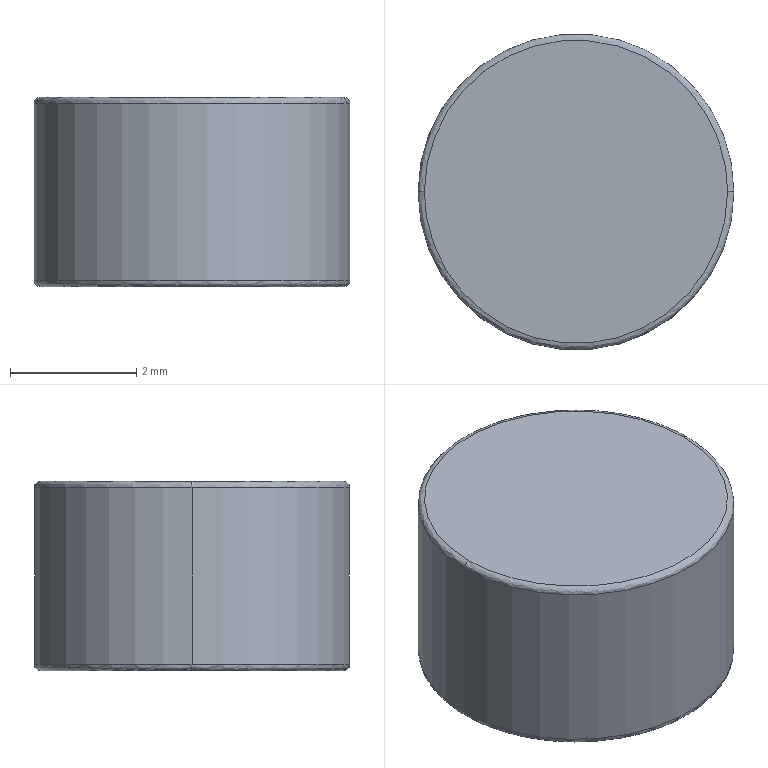Part | SolidWorks | features BaseBody 1 | 1 solid | 8 faces | box 5 x 5 x 3 mm | volume 58.841 mm3 | spline 4 | cylinder 2 | plane 2 | commonest cylinder face diameters 5 x2
STEP:
#1=CARTESIAN_POINT('',(-2.5,0.,0.1));
#2=VERTEX_POINT('',#1);
#3=CARTESIAN_POINT('',(2.5,0.,0.1));
#4=VERTEX_POINT('',#3);
#5=CARTESIAN_POINT('',(0.,0.,0.1));
#6=DIRECTION('',(0.,0.,1.));
#7=DIRECTION('',(-1.,0.,0.));
#8=AXIS2_PLACEMENT_3D('',#5,#6,#7);
#9=CIRCLE('',#8,2.5);
#10=EDGE_CURVE('',#2,#4,#9,.T.);
#11=ORIENTED_EDGE('',*,*,#10,.F.);
#12=CARTESIAN_POINT('',(-2.4,0.,0.));
#13=VERTEX_POINT('',#12);
#14=CARTESIAN_POINT('',(-2.4,0.,0.1));
#15=DIRECTION('',(0.,-1.,0.));
#16=DIRECTION('',(-1.,0.,0.));
#17=AXIS2_PLACEMENT_3D('',#14,#15,#16);
#18=CIRCLE('',#17,0.1);
#19=EDGE_CURVE('',#2,#13,#18,.T.);
#20=ORIENTED_EDGE('',*,*,#19,.T.);
#21=CARTESIAN_POINT('',(2.4,0.,0.));
#22=VERTEX_POINT('',#21);
#23=CARTESIAN_POINT('',(-2.4,0.,0.));
#24=CARTESIAN_POINT('',(-2.4,-4.8,0.));
#25=CARTESIAN_POINT('',(2.4,-4.8,0.));
#26=CARTESIAN_POINT('',(2.4,0.,0.));
#27=(BOUNDED_CURVE()B_SPLINE_CURVE(3,(#23,#24,#25,#26),.UNSPECIFIED.,.F.,.T.)B_SPLINE_CURVE_WITH_KNOTS((4,4),(0.,1.),.UNSPECIFIED.)CURVE()GEOMETRIC_REPRESENTATION_ITEM()RATIONAL_B_SPLINE_CURVE((1.,0.3333,0.3333,1.))REPRESENTATION_ITEM(''));
#28=EDGE_CURVE('',#13,#22,#27,.T.);
#29=ORIENTED_EDGE('',*,*,#28,.T.);
#30=CARTESIAN_POINT('',(2.4,0.,0.1));
#31=DIRECTION('',(0.,1.,0.));
#32=DIRECTION('',(1.,0.,0.));
#33=AXIS2_PLACEMENT_3D('',#30,#31,#32);
#34=CIRCLE('',#33,0.1);
#35=EDGE_CURVE('',#4,#22,#34,.T.);
#36=ORIENTED_EDGE('',*,*,#35,.F.);
#37=EDGE_LOOP('',(#11,#20,#29,#36));
#38=FACE_OUTER_BOUND('',#37,.T.);
#39=CARTESIAN_POINT('',(-2.5,0.,0.1));
#40=CARTESIAN_POINT('',(-2.5,-5.,0.1));
#41=CARTESIAN_POINT('',(2.5,-5.,0.1));
#42=CARTESIAN_POINT('',(2.5,0.,0.1));
#43=CARTESIAN_POINT('',(-2.5,0.,0.04142));
#44=CARTESIAN_POINT('',(-2.5,-5.,0.04142));
#45=CARTESIAN_POINT('',(2.5,-5.,0.04142));
#46=CARTESIAN_POINT('',(2.5,0.,0.04142));
#47=CARTESIAN_POINT('',(-2.459,0.,0.));
#48=CARTESIAN_POINT('',(-2.459,-4.917,0.));
#49=CARTESIAN_POINT('',(2.459,-4.917,0.));
#50=CARTESIAN_POINT('',(2.459,0.,0.));
#51=CARTESIAN_POINT('',(-2.4,0.,0.));
#52=CARTESIAN_POINT('',(-2.4,-4.8,0.));
#53=CARTESIAN_POINT('',(2.4,-4.8,0.));
#54=CARTESIAN_POINT('',(2.4,0.,0.));
#55=(BOUNDED_SURFACE()B_SPLINE_SURFACE(3,3,((#39,#40,#41,#42),(#43,#44,#45,#46),(#47,#48,#49,#50),(#51,#52,#53,#54)),.UNSPECIFIED.,.F.,.F.,.T.)B_SPLINE_SURFACE_WITH_KNOTS((4,4),(4,4),(0.,1.),(0.,1.),.UNSPECIFIED.)GEOMETRIC_REPRESENTATION_ITEM()RATIONAL_B_SPLINE_SURFACE(((1.,0.3333,0.3333,1.),(0.8047,0.2682,0.2682,0.8047),(0.8047,0.2682,0.2682,0.8047),(1.,0.3333,0.3333,1.)))REPRESENTATION_ITEM('')SURFACE());
#56=ADVANCED_FACE('',(#38),#55,.T.);
#57=CARTESIAN_POINT('',(2.4,0.,3.));
#58=VERTEX_POINT('',#57);
#59=CARTESIAN_POINT('',(-2.4,0.,3.));
#60=VERTEX_POINT('',#59);
#61=CARTESIAN_POINT('',(2.4,0.,3.));
#62=CARTESIAN_POINT('',(2.4,-4.8,3.));
#63=CARTESIAN_POINT('',(-2.4,-4.8,3.));
#64=CARTESIAN_POINT('',(-2.4,0.,3.));
#65=(BOUNDED_CURVE()B_SPLINE_CURVE(3,(#61,#62,#63,#64),.UNSPECIFIED.,.F.,.T.)B_SPLINE_CURVE_WITH_KNOTS((4,4),(0.,1.),.UNSPECIFIED.)CURVE()GEOMETRIC_REPRESENTATION_ITEM()RATIONAL_B_SPLINE_CURVE((1.,0.3333,0.3333,1.))REPRESENTATION_ITEM(''));
#66=EDGE_CURVE('',#58,#60,#65,.T.);
#67=ORIENTED_EDGE('',*,*,#66,.T.);
#68=CARTESIAN_POINT('',(-2.5,0.,2.9));
#69=VERTEX_POINT('',#68);
#70=CARTESIAN_POINT('',(-2.4,0.,2.9));
#71=DIRECTION('',(0.,-1.,0.));
#72=DIRECTION('',(-1.,0.,0.));
#73=AXIS2_PLACEMENT_3D('',#70,#71,#72);
#74=CIRCLE('',#73,0.1);
#75=EDGE_CURVE('',#60,#69,#74,.T.);
#76=ORIENTED_EDGE('',*,*,#75,.T.);
#77=CARTESIAN_POINT('',(2.5,0.,2.9));
#78=VERTEX_POINT('',#77);
#79=CARTESIAN_POINT('',(0.,0.,2.9));
#80=DIRECTION('',(0.,0.,-1.));
#81=DIRECTION('',(-1.,0.,0.));
#82=AXIS2_PLACEMENT_3D('',#79,#80,#81);
#83=CIRCLE('',#82,2.5);
#84=EDGE_CURVE('',#78,#69,#83,.T.);
#85=ORIENTED_EDGE('',*,*,#84,.F.);
#86=CARTESIAN_POINT('',(2.4,0.,2.9));
#87=DIRECTION('',(0.,1.,0.));
#88=DIRECTION('',(1.,0.,0.));
#89=AXIS2_PLACEMENT_3D('',#86,#87,#88);
#90=CIRCLE('',#89,0.1);
#91=EDGE_CURVE('',#58,#78,#90,.T.);
#92=ORIENTED_EDGE('',*,*,#91,.F.);
#93=EDGE_LOOP('',(#67,#76,#85,#92));
#94=FACE_OUTER_BOUND('',#93,.T.);
#95=CARTESIAN_POINT('',(-2.4,0.,3.));
#96=CARTESIAN_POINT('',(-2.4,-4.8,3.));
#97=CARTESIAN_POINT('',(2.4,-4.8,3.));
#98=CARTESIAN_POINT('',(2.4,0.,3.));
#99=CARTESIAN_POINT('',(-2.459,0.,3.));
#100=CARTESIAN_POINT('',(-2.459,-4.917,3.));
#101=CARTESIAN_POINT('',(2.459,-4.917,3.));
#102=CARTESIAN_POINT('',(2.459,0.,3.));
#103=CARTESIAN_POINT('',(-2.5,0.,2.959));
#104=CARTESIAN_POINT('',(-2.5,-5.,2.959));
#105=CARTESIAN_POINT('',(2.5,-5.,2.959));
#106=CARTESIAN_POINT('',(2.5,0.,2.959));
#107=CARTESIAN_POINT('',(-2.5,0.,2.9));
#108=CARTESIAN_POINT('',(-2.5,-5.,2.9));
#109=CARTESIAN_POINT('',(2.5,-5.,2.9));
#110=CARTESIAN_POINT('',(2.5,0.,2.9));
#111=(BOUNDED_SURFACE()B_SPLINE_SURFACE(3,3,((#95,#96,#97,#98),(#99,#100,#101,#102),(#103,#104,#105,#106),(#107,#108,#109,#110)),.UNSPECIFIED.,.F.,.F.,.T.)B_SPLINE_SURFACE_WITH_KNOTS((4,4),(4,4),(0.,1.),(0.,1.),.UNSPECIFIED.)GEOMETRIC_REPRESENTATION_ITEM()RATIONAL_B_SPLINE_SURFACE(((1.,0.3333,0.3333,1.),(0.8047,0.2682,0.2682,0.8047),(0.8047,0.2682,0.2682,0.8047),(1.,0.3333,0.3333,1.)))REPRESENTATION_ITEM('')SURFACE());
#112=ADVANCED_FACE('',(#94),#111,.T.);
#113=CARTESIAN_POINT('',(0.,0.,2.9));
#114=DIRECTION('',(0.,0.,-1.));
#115=DIRECTION('',(-1.,0.,0.));
#116=AXIS2_PLACEMENT_3D('',#113,#114,#115);
#117=CIRCLE('',#116,2.5);
#118=EDGE_CURVE('',#69,#78,#117,.T.);
#119=ORIENTED_EDGE('',*,*,#118,.T.);
#120=CARTESIAN_POINT('',(2.5,0.,3.));
#121=DIRECTION('',(0.,0.,-1.));
#122=VECTOR('',#121,1000.);
#123=LINE('',#120,#122);
#124=EDGE_CURVE('',#78,#4,#123,.T.);
#125=ORIENTED_EDGE('',*,*,#124,.T.);
#126=CARTESIAN_POINT('',(0.,0.,0.1));
#127=DIRECTION('',(0.,0.,1.));
#128=DIRECTION('',(-1.,0.,0.));
#129=AXIS2_PLACEMENT_3D('',#126,#127,#128);
#130=CIRCLE('',#129,2.5);
#131=EDGE_CURVE('',#4,#2,#130,.T.);
#132=ORIENTED_EDGE('',*,*,#131,.T.);
#133=CARTESIAN_POINT('',(-2.5,0.,3.));
#134=DIRECTION('',(0.,0.,-1.));
#135=VECTOR('',#134,1000.);
#136=LINE('',#133,#135);
#137=EDGE_CURVE('',#69,#2,#136,.T.);
#138=ORIENTED_EDGE('',*,*,#137,.F.);
#139=EDGE_LOOP('',(#119,#125,#132,#138));
#140=FACE_OUTER_BOUND('',#139,.T.);
#141=CARTESIAN_POINT('',(0.,0.,3.));
#142=DIRECTION('',(0.,0.,-1.));
#143=DIRECTION('',(-1.,0.,0.));
#144=AXIS2_PLACEMENT_3D('',#141,#142,#143);
#145=CYLINDRICAL_SURFACE('',#144,2.5);
#146=ADVANCED_FACE('',(#140),#145,.T.);
#147=ORIENTED_EDGE('',*,*,#124,.F.);
#148=ORIENTED_EDGE('',*,*,#84,.T.);
#149=ORIENTED_EDGE('',*,*,#137,.T.);
#150=ORIENTED_EDGE('',*,*,#10,.T.);
#151=EDGE_LOOP('',(#147,#148,#149,#150));
#152=FACE_OUTER_BOUND('',#151,.T.);
#153=CARTESIAN_POINT('',(0.,0.,3.));
#154=DIRECTION('',(0.,0.,-1.));
#155=DIRECTION('',(-1.,0.,0.));
#156=AXIS2_PLACEMENT_3D('',#153,#154,#155);
#157=CYLINDRICAL_SURFACE('',#156,2.5);
#158=ADVANCED_FACE('',(#152),#157,.T.);
#159=ORIENTED_EDGE('',*,*,#19,.F.);
#160=ORIENTED_EDGE('',*,*,#131,.F.);
#161=ORIENTED_EDGE('',*,*,#35,.T.);
#162=CARTESIAN_POINT('',(2.4,0.,0.));
#163=CARTESIAN_POINT('',(2.4,4.8,0.));
#164=CARTESIAN_POINT('',(-2.4,4.8,0.));
#165=CARTESIAN_POINT('',(-2.4,0.,0.));
#166=(BOUNDED_CURVE()B_SPLINE_CURVE(3,(#162,#163,#164,#165),.UNSPECIFIED.,.F.,.T.)B_SPLINE_CURVE_WITH_KNOTS((4,4),(0.,1.),.UNSPECIFIED.)CURVE()GEOMETRIC_REPRESENTATION_ITEM()RATIONAL_B_SPLINE_CURVE((1.,0.3333,0.3333,1.))REPRESENTATION_ITEM(''));
#167=EDGE_CURVE('',#22,#13,#166,.T.);
#168=ORIENTED_EDGE('',*,*,#167,.T.);
#169=EDGE_LOOP('',(#159,#160,#161,#168));
#170=FACE_OUTER_BOUND('',#169,.T.);
#171=CARTESIAN_POINT('',(2.5,0.,0.1));
#172=CARTESIAN_POINT('',(2.5,5.,0.1));
#173=CARTESIAN_POINT('',(-2.5,5.,0.1));
#174=CARTESIAN_POINT('',(-2.5,0.,0.1));
#175=CARTESIAN_POINT('',(2.5,0.,0.04142));
#176=CARTESIAN_POINT('',(2.5,5.,0.04142));
#177=CARTESIAN_POINT('',(-2.5,5.,0.04142));
#178=CARTESIAN_POINT('',(-2.5,0.,0.04142));
#179=CARTESIAN_POINT('',(2.459,0.,0.));
#180=CARTESIAN_POINT('',(2.459,4.917,0.));
#181=CARTESIAN_POINT('',(-2.459,4.917,0.));
#182=CARTESIAN_POINT('',(-2.459,0.,0.));
#183=CARTESIAN_POINT('',(2.4,0.,0.));
#184=CARTESIAN_POINT('',(2.4,4.8,0.));
#185=CARTESIAN_POINT('',(-2.4,4.8,0.));
#186=CARTESIAN_POINT('',(-2.4,0.,0.));
#187=(BOUNDED_SURFACE()B_SPLINE_SURFACE(3,3,((#171,#172,#173,#174),(#175,#176,#177,#178),(#179,#180,#181,#182),(#183,#184,#185,#186)),.UNSPECIFIED.,.F.,.F.,.T.)B_SPLINE_SURFACE_WITH_KNOTS((4,4),(4,4),(0.,1.),(0.,1.),.UNSPECIFIED.)GEOMETRIC_REPRESENTATION_ITEM()RATIONAL_B_SPLINE_SURFACE(((1.,0.3333,0.3333,1.),(0.8047,0.2682,0.2682,0.8047),(0.8047,0.2682,0.2682,0.8047),(1.,0.3333,0.3333,1.)))REPRESENTATION_ITEM('')SURFACE());
#188=ADVANCED_FACE('',(#170),#187,.T.);
#189=ORIENTED_EDGE('',*,*,#75,.F.);
#190=CARTESIAN_POINT('',(-2.4,0.,3.));
#191=CARTESIAN_POINT('',(-2.4,4.8,3.));
#192=CARTESIAN_POINT('',(2.4,4.8,3.));
#193=CARTESIAN_POINT('',(2.4,0.,3.));
#194=(BOUNDED_CURVE()B_SPLINE_CURVE(3,(#190,#191,#192,#193),.UNSPECIFIED.,.F.,.T.)B_SPLINE_CURVE_WITH_KNOTS((4,4),(0.,1.),.UNSPECIFIED.)CURVE()GEOMETRIC_REPRESENTATION_ITEM()RATIONAL_B_SPLINE_CURVE((1.,0.3333,0.3333,1.))REPRESENTATION_ITEM(''));
#195=EDGE_CURVE('',#60,#58,#194,.T.);
#196=ORIENTED_EDGE('',*,*,#195,.T.);
#197=ORIENTED_EDGE('',*,*,#91,.T.);
#198=ORIENTED_EDGE('',*,*,#118,.F.);
#199=EDGE_LOOP('',(#189,#196,#197,#198));
#200=FACE_OUTER_BOUND('',#199,.T.);
#201=CARTESIAN_POINT('',(2.4,0.,3.));
#202=CARTESIAN_POINT('',(2.4,4.8,3.));
#203=CARTESIAN_POINT('',(-2.4,4.8,3.));
#204=CARTESIAN_POINT('',(-2.4,0.,3.));
#205=CARTESIAN_POINT('',(2.459,0.,3.));
#206=CARTESIAN_POINT('',(2.459,4.917,3.));
#207=CARTESIAN_POINT('',(-2.459,4.917,3.));
#208=CARTESIAN_POINT('',(-2.459,0.,3.));
#209=CARTESIAN_POINT('',(2.5,0.,2.959));
#210=CARTESIAN_POINT('',(2.5,5.,2.959));
#211=CARTESIAN_POINT('',(-2.5,5.,2.959));
#212=CARTESIAN_POINT('',(-2.5,0.,2.959));
#213=CARTESIAN_POINT('',(2.5,0.,2.9));
#214=CARTESIAN_POINT('',(2.5,5.,2.9));
#215=CARTESIAN_POINT('',(-2.5,5.,2.9));
#216=CARTESIAN_POINT('',(-2.5,0.,2.9));
#217=(BOUNDED_SURFACE()B_SPLINE_SURFACE(3,3,((#201,#202,#203,#204),(#205,#206,#207,#208),(#209,#210,#211,#212),(#213,#214,#215,#216)),.UNSPECIFIED.,.F.,.F.,.F.)B_SPLINE_SURFACE_WITH_KNOTS((4,4),(4,4),(0.,1.),(0.,1.),.UNSPECIFIED.)GEOMETRIC_REPRESENTATION_ITEM()RATIONAL_B_SPLINE_SURFACE(((1.,0.3333,0.3333,1.),(0.8047,0.2682,0.2682,0.8047),(0.8047,0.2682,0.2682,0.8047),(1.,0.3333,0.3333,1.)))REPRESENTATION_ITEM('')SURFACE());
#218=ADVANCED_FACE('',(#200),#217,.T.);
#219=ORIENTED_EDGE('',*,*,#167,.F.);
#220=ORIENTED_EDGE('',*,*,#28,.F.);
#221=EDGE_LOOP('',(#219,#220));
#222=FACE_OUTER_BOUND('',#221,.T.);
#223=CARTESIAN_POINT('',(0.,0.,0.));
#224=DIRECTION('',(0.,0.,1.));
#225=DIRECTION('',(1.,0.,0.));
#226=AXIS2_PLACEMENT_3D('',#223,#224,#225);
#227=PLANE('',#226);
#228=ADVANCED_FACE('',(#222),#227,.F.);
#229=ORIENTED_EDGE('',*,*,#195,.F.);
#230=ORIENTED_EDGE('',*,*,#66,.F.);
#231=EDGE_LOOP('',(#229,#230));
#232=FACE_OUTER_BOUND('',#231,.T.);
#233=CARTESIAN_POINT('',(0.,0.,3.));
#234=DIRECTION('',(0.,0.,1.));
#235=DIRECTION('',(1.,0.,0.));
#236=AXIS2_PLACEMENT_3D('',#233,#234,#235);
#237=PLANE('',#236);
#238=ADVANCED_FACE('',(#232),#237,.T.);
#239=CLOSED_SHELL('',(#56,#112,#146,#158,#188,#218,#228,#238));
#240=MANIFOLD_SOLID_BREP('',#239);
#241=CARTESIAN_POINT('',(0.,0.,0.));
#242=DIRECTION('',(0.,0.,1.));
#243=DIRECTION('',(1.,0.,0.));
#244=AXIS2_PLACEMENT_3D('',#241,#242,#243);
#245=(LENGTH_UNIT()NAMED_UNIT(*)SI_UNIT(.MILLI.,.METRE.));
#246=UNCERTAINTY_MEASURE_WITH_UNIT(LENGTH_MEASURE(0.00001),#245,'','');
#247=(NAMED_UNIT(*)PLANE_ANGLE_UNIT()SI_UNIT($,.RADIAN.));
#248=(NAMED_UNIT(*)SI_UNIT($,.STERADIAN.)SOLID_ANGLE_UNIT());
#249=(GEOMETRIC_REPRESENTATION_CONTEXT(3)GLOBAL_UNCERTAINTY_ASSIGNED_CONTEXT((#246))GLOBAL_UNIT_ASSIGNED_CONTEXT((#245,#247,#248))REPRESENTATION_CONTEXT('',''));
#250=ADVANCED_BREP_SHAPE_REPRESENTATION('',(#240,#244),#249);